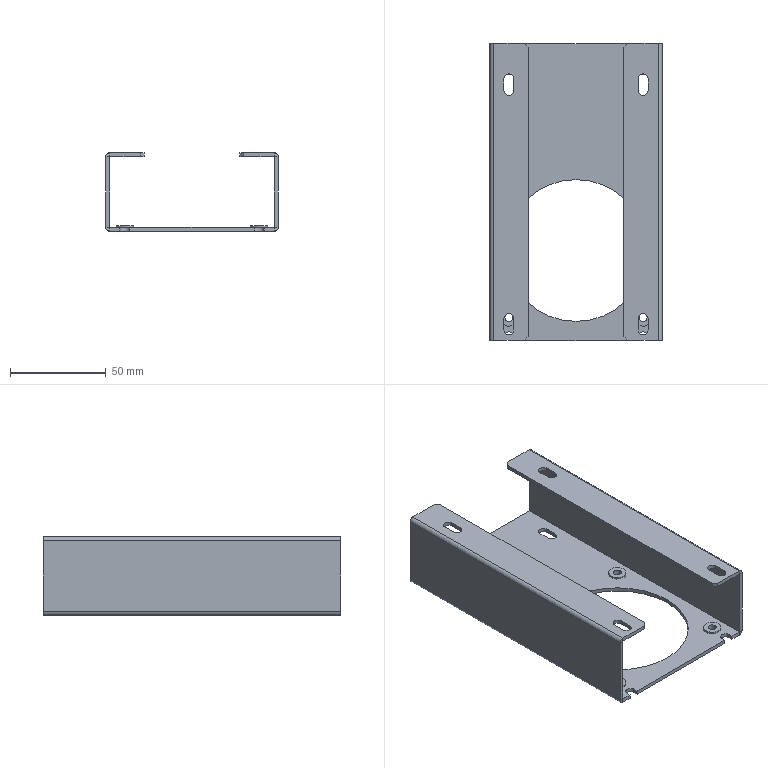Part | STEP file | 86 motor mounting flange | 1 solid | 96 faces | box 90 x 155 x 41 mm | volume 53412 mm3 | plane 56 | cylinder 40 | commonest cylinder face diameters 5.2 x14 4.2 x12 9 x8 0.2 x4 74 x2